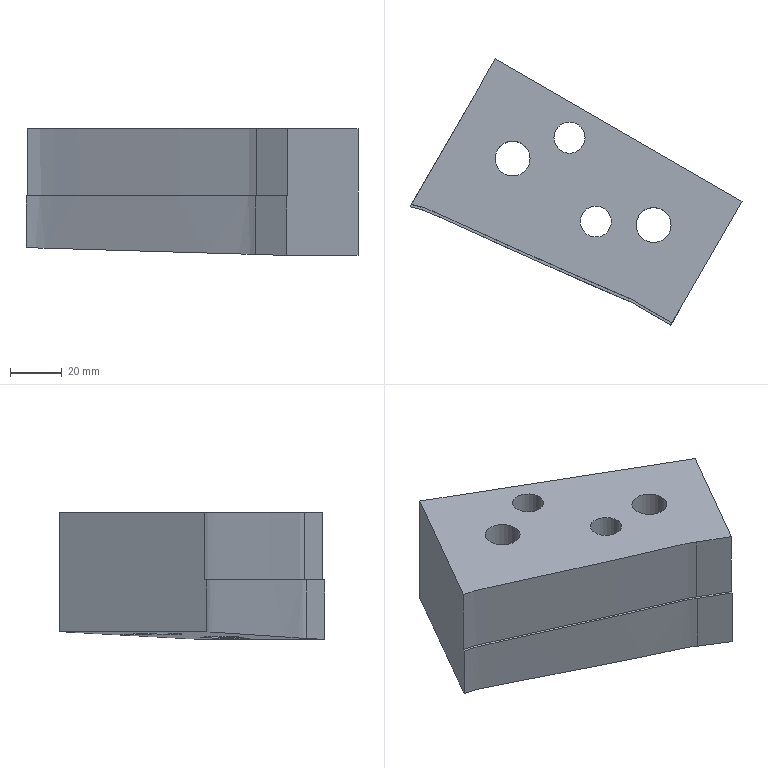Part | NX | features solid 2 | 1 solid | 22 faces | box 128.226 x 102.703 x 49 mm | volume 276802 mm3 | plane 12 | cylinder 8 | spline 2 | commonest cylinder face diameters 12 x2 13 x2 13.5 x2 19.5 x2
STEP:
#1=CARTESIAN_POINT('',(308.582,133.358,14.));
#2=VERTEX_POINT('',#1);
#3=CARTESIAN_POINT('',(397.207,94.712,14.));
#4=VERTEX_POINT('',#3);
#5=CARTESIAN_POINT('',(-190.231,-121.49,14.));
#6=CARTESIAN_POINT('',(-188.654,-121.152,14.));
#7=CARTESIAN_POINT('',(-185.47,-120.627,14.));
#8=CARTESIAN_POINT('',(-180.656,-120.141,14.));
#9=CARTESIAN_POINT('',(-175.882,-119.326,14.));
#10=CARTESIAN_POINT('',(-169.679,-117.528,14.));
#11=CARTESIAN_POINT('',(-162.185,-114.539,14.));
#12=CARTESIAN_POINT('',(-153.086,-111.254,14.));
#13=CARTESIAN_POINT('',(-144.031,-107.845,14.));
#14=CARTESIAN_POINT('',(-136.465,-105.061,14.));
#15=CARTESIAN_POINT('',(-130.418,-102.814,14.));
#16=CARTESIAN_POINT('',(-125.812,-101.329,14.));
#17=CARTESIAN_POINT('',(-121.306,-99.566,14.));
#18=CARTESIAN_POINT('',(-116.876,-97.626,14.));
#19=CARTESIAN_POINT('',(-112.335,-95.923,14.));
#20=CARTESIAN_POINT('',(-107.564,-95.05,14.));
#21=CARTESIAN_POINT('',(-102.756,-94.525,14.));
#22=CARTESIAN_POINT('',(-96.349,-93.771,14.));
#23=CARTESIAN_POINT('',(-89.902,-93.468,14.));
#24=CARTESIAN_POINT('',(-83.452,-93.448,14.));
#25=CARTESIAN_POINT('',(-77.002,-93.469,14.));
#26=CARTESIAN_POINT('',(-68.939,-93.411,14.));
#27=CARTESIAN_POINT('',(-56.04,-93.3,14.));
#28=CARTESIAN_POINT('',(-33.465,-93.184,14.));
#29=CARTESIAN_POINT('',(-7.666,-93.074,14.));
#30=CARTESIAN_POINT('',(14.907,-92.653,14.));
#31=CARTESIAN_POINT('',(27.794,-92.068,14.));
#32=CARTESIAN_POINT('',(40.668,-91.245,14.));
#33=CARTESIAN_POINT('',(51.917,-90.291,14.));
#34=CARTESIAN_POINT('',(61.528,-89.174,14.));
#35=CARTESIAN_POINT('',(67.939,-88.466,14.));
#36=CARTESIAN_POINT('',(79.125,-86.95,14.));
#37=CARTESIAN_POINT('',(95.161,-85.253,14.));
#38=CARTESIAN_POINT('',(114.404,-83.21,14.));
#39=CARTESIAN_POINT('',(133.568,-80.524,14.));
#40=CARTESIAN_POINT('',(152.734,-77.861,14.));
#41=CARTESIAN_POINT('',(171.916,-75.326,14.));
#42=CARTESIAN_POINT('',(191.055,-72.413,14.));
#43=CARTESIAN_POINT('',(207.17,-71.468,14.));
#44=CARTESIAN_POINT('',(219.951,-69.697,14.));
#45=CARTESIAN_POINT('',(232.724,-67.899,14.));
#46=CARTESIAN_POINT('',(248.708,-65.766,14.));
#47=CARTESIAN_POINT('',(267.87,-63.074,14.));
#48=CARTESIAN_POINT('',(287.038,-60.44,14.));
#49=CARTESIAN_POINT('',(301.448,-58.682,14.));
#50=CARTESIAN_POINT('',(310.976,-56.987,14.));
#51=CARTESIAN_POINT('',(314.916,-56.135,14.));
#52=CARTESIAN_POINT('',(318.052,-55.382,14.));
#53=CARTESIAN_POINT('',(320.39,-54.76,14.));
#54=CARTESIAN_POINT('',(322.686,-53.981,14.));
#55=CARTESIAN_POINT('',(325.595,-52.578,14.));
#56=CARTESIAN_POINT('',(328.769,-50.098,14.));
#57=CARTESIAN_POINT('',(332.247,-46.69,14.));
#58=CARTESIAN_POINT('',(335.795,-43.406,14.));
#59=CARTESIAN_POINT('',(343.661,-37.758,14.));
#60=CARTESIAN_POINT('',(355.164,-28.914,14.));
#61=CARTESIAN_POINT('',(370.422,-17.018,14.));
#62=CARTESIAN_POINT('',(383.264,-7.249,14.));
#63=CARTESIAN_POINT('',(392.416,-0.6713,14.));
#64=CARTESIAN_POINT('',(396.953,2.733,14.));
#65=CARTESIAN_POINT('',(398.886,5.372,14.));
#66=CARTESIAN_POINT('',(399.725,7.654,14.));
#67=CARTESIAN_POINT('',(399.76,10.078,14.));
#68=CARTESIAN_POINT('',(399.483,13.317,14.));
#69=CARTESIAN_POINT('',(399.712,17.34,14.));
#70=CARTESIAN_POINT('',(399.612,22.179,14.));
#71=CARTESIAN_POINT('',(399.633,31.854,14.));
#72=CARTESIAN_POINT('',(399.593,46.366,14.));
#73=CARTESIAN_POINT('',(399.637,62.491,14.));
#74=CARTESIAN_POINT('',(399.588,73.779,14.));
#75=CARTESIAN_POINT('',(399.652,79.422,14.));
#76=CARTESIAN_POINT('',(399.59,82.647,14.));
#77=CARTESIAN_POINT('',(399.564,85.065,14.));
#78=CARTESIAN_POINT('',(399.725,87.486,14.));
#79=CARTESIAN_POINT('',(399.756,89.902,14.));
#80=CARTESIAN_POINT('',(399.247,92.301,14.));
#81=CARTESIAN_POINT('',(397.362,95.008,14.));
#82=CARTESIAN_POINT('',(393.635,96.774,14.));
#83=CARTESIAN_POINT('',(389.279,98.826,14.));
#84=CARTESIAN_POINT('',(384.732,100.498,14.));
#85=CARTESIAN_POINT('',(378.765,102.95,14.));
#86=CARTESIAN_POINT('',(362.589,110.229,14.));
#87=CARTESIAN_POINT('',(344.928,118.135,14.));
#88=CARTESIAN_POINT('',(327.281,126.072,14.));
#89=CARTESIAN_POINT('',(319.932,129.381,14.));
#90=CARTESIAN_POINT('',(314.075,132.102,14.));
#91=CARTESIAN_POINT('',(309.387,133.376,14.));
#92=CARTESIAN_POINT('',(304.547,133.785,14.));
#93=CARTESIAN_POINT('',(299.716,133.401,14.));
#94=CARTESIAN_POINT('',(294.929,132.704,14.));
#95=CARTESIAN_POINT('',(288.543,131.8,14.));
#96=CARTESIAN_POINT('',(277.364,130.241,14.));
#97=CARTESIAN_POINT('',(242.2,125.552,14.));
#98=CARTESIAN_POINT('',(184.637,118.048,14.));
#99=CARTESIAN_POINT('',(120.701,109.541,14.));
#100=CARTESIAN_POINT('',(69.531,102.902,14.));
#101=CARTESIAN_POINT('',(40.777,98.94,14.));
#102=CARTESIAN_POINT('',(21.566,96.615,14.));
#103=CARTESIAN_POINT('',(8.743,95.212,14.));
#104=CARTESIAN_POINT('',(-7.301,93.575,14.));
#105=CARTESIAN_POINT('',(-26.625,92.505,14.));
#106=CARTESIAN_POINT('',(-45.971,92.017,14.));
#107=CARTESIAN_POINT('',(-62.09,91.675,14.));
#108=CARTESIAN_POINT('',(-74.987,91.256,14.));
#109=CARTESIAN_POINT('',(-84.664,91.165,14.));
#110=CARTESIAN_POINT('',(-94.319,91.781,14.));
#111=CARTESIAN_POINT('',(-103.929,92.966,14.));
#112=CARTESIAN_POINT('',(-113.495,94.403,14.));
#113=CARTESIAN_POINT('',(-119.856,95.492,14.));
#114=CARTESIAN_POINT('',(-122.997,96.222,14.));
#115=B_SPLINE_CURVE_WITH_KNOTS('',3,(#5,#6,#7,#8,#9,#10,#11,#12,#13,#14,#15,#16,#17,#18,#19,#20,#21,#22,#23,#24,#25,#26,#27,#28,#29,#30,#31,#32,#33,#34,#35,#36,#37,#38,#39,#40,#41,#42,#43,#44,#45,#46,#47,#48,#49,#50,#51,#52,#53,#54,#55,#56,#57,#58,#59,#60,#61,#62,#63,#64,#65,#66,#67,#68,#69,#70,#71,#72,#73,#74,#75,#76,#77,#78,#79,#80,#81,#82,#83,#84,#85,#86,#87,#88,#89,#90,#91,#92,#93,#94,#95,#96,#97,#98,#99,#100,#101,#102,#103,#104,#105,#106,#107,#108,#109,#110,#111,#112,#113,#114),.UNSPECIFIED.,.F.,.F.,(4,1,1,1,1,1,1,1,1,1,1,1,1,1,1,1,1,1,1,1,1,1,1,1,1,1,1,1,1,1,1,1,1,1,1,1,1,1,1,1,1,1,1,1,1,1,1,1,1,1,1,1,1,1,1,1,1,1,1,1,1,1,1,1,1,1,1,1,1,1,1,1,1,1,1,1,1,1,1,1,1,1,1,1,1,1,1,1,1,1,1,1,1,1,1,1,1,1,1,1,1,1,1,1,1,1,1,4),(0.4704,0.4724,0.4745,0.4766,0.4786,0.4828,0.4869,0.491,0.4952,0.4972,0.4993,0.5014,0.5035,0.5055,0.5076,0.5097,0.5117,0.5159,0.5179,0.52,0.5241,0.5283,0.5366,0.5531,0.5614,0.5655,0.5697,0.5779,0.58,0.5821,0.5862,0.5945,0.6028,0.611,0.6193,0.6276,0.6359,0.6441,0.6483,0.6524,0.6607,0.669,0.6772,0.6855,0.6876,0.6897,0.6907,0.6917,0.6928,0.6938,0.6959,0.6979,0.7,0.7021,0.7103,0.7186,0.7269,0.731,0.7331,0.7341,0.7352,0.7362,0.7372,0.7393,0.7414,0.7435,0.7517,0.76,0.7641,0.7662,0.7672,0.7683,0.7693,0.7703,0.7714,0.7724,0.7745,0.7766,0.7786,0.7807,0.7848,0.8014,0.8055,0.8097,0.8117,0.8138,0.8159,0.8179,0.82,0.8221,0.8262,0.8345,0.8676,0.9007,0.9172,0.9338,0.9379,0.9421,0.9503,0.9586,0.9669,0.9752,0.9793,0.9834,0.9876,0.9917,0.9959,1.),.UNSPECIFIED.);
#116=EDGE_CURVE('',#2,#4,#115,.F.);
#117=ORIENTED_EDGE('',*,*,#116,.F.);
#118=CARTESIAN_POINT('',(308.582,133.358,-6.));
#119=VERTEX_POINT('',#118);
#120=CARTESIAN_POINT('',(308.582,133.358,4.));
#121=DIRECTION('',(0.,0.,-1.));
#122=VECTOR('',#121,1000.);
#123=LINE('',#120,#122);
#124=EDGE_CURVE('',#119,#2,#123,.F.);
#125=ORIENTED_EDGE('',*,*,#124,.F.);
#126=CARTESIAN_POINT('',(397.207,94.712,-8.62));
#127=VERTEX_POINT('',#126);
#128=CARTESIAN_POINT('',(308.582,133.358,-6.));
#129=CARTESIAN_POINT('',(310.591,133.063,-6.051));
#130=CARTESIAN_POINT('',(314.461,132.008,-6.157));
#131=CARTESIAN_POINT('',(321.748,128.497,-6.377));
#132=CARTESIAN_POINT('',(330.972,124.433,-6.651));
#133=CARTESIAN_POINT('',(342.006,119.447,-6.979));
#134=CARTESIAN_POINT('',(353.053,114.5,-7.308));
#135=CARTESIAN_POINT('',(362.257,110.369,-7.581));
#136=CARTESIAN_POINT('',(369.619,107.065,-7.8));
#137=CARTESIAN_POINT('',(375.138,104.579,-7.964));
#138=CARTESIAN_POINT('',(380.676,102.138,-8.129));
#139=CARTESIAN_POINT('',(385.367,100.278,-8.265));
#140=CARTESIAN_POINT('',(389.141,98.841,-8.373));
#141=CARTESIAN_POINT('',(391.899,97.59,-8.456));
#142=CARTESIAN_POINT('',(394.641,96.327,-8.538));
#143=CARTESIAN_POINT('',(396.433,95.353,-8.593));
#144=CARTESIAN_POINT('',(397.207,94.712,-8.62));
#145=B_SPLINE_CURVE_WITH_KNOTS('',3,(#128,#129,#130,#131,#132,#133,#134,#135,#136,#137,#138,#139,#140,#141,#142,#143,#144),.UNSPECIFIED.,.F.,.F.,(4,1,1,1,1,1,1,1,1,1,1,1,1,1,4),(0.,0.006012,0.01202,0.02405,0.03607,0.0481,0.06012,0.06613,0.07214,0.07816,0.08417,0.08717,0.09018,0.09319,0.09619),.UNSPECIFIED.);
#146=EDGE_CURVE('',#119,#127,#145,.T.);
#147=ORIENTED_EDGE('',*,*,#146,.T.);
#148=CARTESIAN_POINT('',(397.207,94.712,15.353));
#149=DIRECTION('',(0.,0.,-1.));
#150=VECTOR('',#149,1000.);
#151=LINE('',#148,#150);
#152=EDGE_CURVE('',#127,#4,#151,.F.);
#153=ORIENTED_EDGE('',*,*,#152,.T.);
#154=EDGE_LOOP('',(#117,#125,#147,#153));
#155=FACE_BOUND('',#154,.T.);
#156=CARTESIAN_POINT('',(397.207,94.712,14.));
#157=CARTESIAN_POINT('',(397.207,94.712,-8.756));
#158=CARTESIAN_POINT('',(396.44,95.348,14.));
#159=CARTESIAN_POINT('',(396.44,95.348,-8.756));
#160=CARTESIAN_POINT('',(394.655,96.321,14.));
#161=CARTESIAN_POINT('',(394.655,96.321,-8.756));
#162=CARTESIAN_POINT('',(391.88,97.598,14.));
#163=CARTESIAN_POINT('',(391.88,97.598,-8.756));
#164=CARTESIAN_POINT('',(389.14,98.841,14.));
#165=CARTESIAN_POINT('',(389.14,98.841,-8.756));
#166=CARTESIAN_POINT('',(385.368,100.277,14.));
#167=CARTESIAN_POINT('',(385.368,100.277,-8.756));
#168=CARTESIAN_POINT('',(380.678,102.137,14.));
#169=CARTESIAN_POINT('',(380.678,102.137,-8.756));
#170=CARTESIAN_POINT('',(375.142,104.577,14.));
#171=CARTESIAN_POINT('',(375.142,104.577,-8.756));
#172=CARTESIAN_POINT('',(369.625,107.062,14.));
#173=CARTESIAN_POINT('',(369.625,107.062,-8.756));
#174=CARTESIAN_POINT('',(362.265,110.366,14.));
#175=CARTESIAN_POINT('',(362.265,110.366,-8.756));
#176=CARTESIAN_POINT('',(353.065,114.495,14.));
#177=CARTESIAN_POINT('',(353.065,114.495,-8.756));
#178=CARTESIAN_POINT('',(342.021,119.44,14.));
#179=CARTESIAN_POINT('',(342.021,119.44,-8.756));
#180=CARTESIAN_POINT('',(330.992,124.425,14.));
#181=CARTESIAN_POINT('',(330.992,124.425,-8.756));
#182=CARTESIAN_POINT('',(321.77,128.484,14.));
#183=CARTESIAN_POINT('',(321.77,128.484,-8.756));
#184=CARTESIAN_POINT('',(314.49,131.999,14.));
#185=CARTESIAN_POINT('',(314.49,131.999,-8.756));
#186=CARTESIAN_POINT('',(310.577,133.065,14.));
#187=CARTESIAN_POINT('',(310.577,133.065,-8.756));
#188=CARTESIAN_POINT('',(308.582,133.358,14.));
#189=CARTESIAN_POINT('',(308.582,133.358,-8.756));
#190=B_SPLINE_SURFACE_WITH_KNOTS('',3,1,((#156,#157),(#158,#159),(#160,#161),(#162,#163),(#164,#165),(#166,#167),(#168,#169),(#170,#171),(#172,#173),(#174,#175),(#176,#177),(#178,#179),(#180,#181),(#182,#183),(#184,#185),(#186,#187),(#188,#189)),.SURF_OF_LINEAR_EXTRUSION.,.F.,.F.,.F.,(4,1,1,1,1,1,1,1,1,1,1,1,1,1,4),(2,2),(0.7727,0.774,0.7753,0.7766,0.7779,0.7805,0.7831,0.7857,0.7883,0.7934,0.7986,0.8038,0.809,0.8115,0.8141),(0.,1.),.UNSPECIFIED.);
#191=ADVANCED_FACE('',(#155),#190,.T.);
#192=CARTESIAN_POINT('',(409.767,88.615,40.));
#193=VERTEX_POINT('',#192);
#194=CARTESIAN_POINT('',(397.778,95.537,40.));
#195=VERTEX_POINT('',#194);
#196=CARTESIAN_POINT('',(-185.99,432.575,40.));
#197=DIRECTION('',(-0.866,0.5,0.));
#198=VECTOR('',#197,1000.);
#199=LINE('',#196,#198);
#200=EDGE_CURVE('',#193,#195,#199,.T.);
#201=ORIENTED_EDGE('',*,*,#200,.F.);
#202=CARTESIAN_POINT('',(436.808,135.452,40.));
#203=VERTEX_POINT('',#202);
#204=CARTESIAN_POINT('',(180.279,-308.87,40.));
#205=DIRECTION('',(0.5,0.866,0.));
#206=VECTOR('',#205,1000.);
#207=LINE('',#204,#206);
#208=EDGE_CURVE('',#193,#203,#207,.T.);
#209=ORIENTED_EDGE('',*,*,#208,.T.);
#210=CARTESIAN_POINT('',(341.545,190.452,40.));
#211=VERTEX_POINT('',#210);
#212=CARTESIAN_POINT('',(-158.948,479.412,40.));
#213=DIRECTION('',(0.866,-0.5,0.));
#214=VECTOR('',#213,1000.);
#215=LINE('',#212,#214);
#216=EDGE_CURVE('',#211,#203,#215,.T.);
#217=ORIENTED_EDGE('',*,*,#216,.F.);
#218=CARTESIAN_POINT('',(309.118,134.287,40.));
#219=VERTEX_POINT('',#218);
#220=CARTESIAN_POINT('',(85.016,-253.87,40.));
#221=DIRECTION('',(0.5,0.866,0.));
#222=VECTOR('',#221,1000.);
#223=LINE('',#220,#222);
#224=EDGE_CURVE('',#219,#211,#223,.T.);
#225=ORIENTED_EDGE('',*,*,#224,.F.);
#226=CARTESIAN_POINT('',(397.778,95.537,40.));
#227=CARTESIAN_POINT('',(396.982,96.183,40.));
#228=CARTESIAN_POINT('',(395.223,97.16,40.));
#229=CARTESIAN_POINT('',(392.476,98.422,40.));
#230=CARTESIAN_POINT('',(389.726,99.681,40.));
#231=CARTESIAN_POINT('',(385.959,101.127,40.));
#232=CARTESIAN_POINT('',(381.266,102.971,40.));
#233=CARTESIAN_POINT('',(375.729,105.41,40.));
#234=CARTESIAN_POINT('',(370.211,107.895,40.));
#235=CARTESIAN_POINT('',(362.85,111.199,40.));
#236=CARTESIAN_POINT('',(353.649,115.329,40.));
#237=CARTESIAN_POINT('',(342.603,120.275,40.));
#238=CARTESIAN_POINT('',(331.573,125.26,40.));
#239=CARTESIAN_POINT('',(322.344,129.323,40.));
#240=CARTESIAN_POINT('',(315.069,132.831,40.));
#241=CARTESIAN_POINT('',(311.167,133.957,40.));
#242=CARTESIAN_POINT('',(309.118,134.287,40.));
#243=B_SPLINE_CURVE_WITH_KNOTS('',3,(#226,#227,#228,#229,#230,#231,#232,#233,#234,#235,#236,#237,#238,#239,#240,#241,#242),.UNSPECIFIED.,.F.,.F.,(4,1,1,1,1,1,1,1,1,1,1,1,1,1,4),(0.009262,0.01231,0.01537,0.01842,0.02147,0.02758,0.03368,0.03979,0.04589,0.0581,0.07031,0.08252,0.09473,0.1008,0.1069),.UNSPECIFIED.);
#244=EDGE_CURVE('',#195,#219,#243,.T.);
#245=ORIENTED_EDGE('',*,*,#244,.F.);
#246=EDGE_LOOP('',(#201,#209,#217,#225,#245));
#247=FACE_BOUND('',#246,.T.);
#248=CARTESIAN_POINT('',(386.337,127.641,40.));
#249=VERTEX_POINT('',#248);
#250=CARTESIAN_POINT('',(380.337,127.641,40.));
#251=DIRECTION('',(0.,0.,1.));
#252=DIRECTION('',(1.,0.,0.));
#253=AXIS2_PLACEMENT_3D('',#250,#251,#252);
#254=CIRCLE('',#253,6.);
#255=EDGE_CURVE('',#249,#249,#254,.T.);
#256=ORIENTED_EDGE('',*,*,#255,.F.);
#257=EDGE_LOOP('',(#256));
#258=FACE_BOUND('',#257,.T.);
#259=CARTESIAN_POINT('',(376.186,160.059,40.));
#260=VERTEX_POINT('',#259);
#261=CARTESIAN_POINT('',(370.186,160.059,40.));
#262=DIRECTION('',(0.,0.,1.));
#263=DIRECTION('',(1.,0.,0.));
#264=AXIS2_PLACEMENT_3D('',#261,#262,#263);
#265=CIRCLE('',#264,6.);
#266=EDGE_CURVE('',#260,#260,#265,.T.);
#267=ORIENTED_EDGE('',*,*,#266,.F.);
#268=EDGE_LOOP('',(#267));
#269=FACE_BOUND('',#268,.T.);
#270=CARTESIAN_POINT('',(409.407,126.301,40.));
#271=VERTEX_POINT('',#270);
#272=CARTESIAN_POINT('',(402.657,126.301,40.));
#273=DIRECTION('',(0.,0.,1.));
#274=DIRECTION('',(1.,0.,0.));
#275=AXIS2_PLACEMENT_3D('',#272,#273,#274);
#276=CIRCLE('',#275,6.75);
#277=EDGE_CURVE('',#271,#271,#276,.T.);
#278=ORIENTED_EDGE('',*,*,#277,.F.);
#279=EDGE_LOOP('',(#278));
#280=FACE_BOUND('',#279,.T.);
#281=CARTESIAN_POINT('',(354.946,151.971,40.));
#282=VERTEX_POINT('',#281);
#283=CARTESIAN_POINT('',(348.196,151.971,40.));
#284=DIRECTION('',(0.,0.,1.));
#285=DIRECTION('',(1.,0.,0.));
#286=AXIS2_PLACEMENT_3D('',#283,#284,#285);
#287=CIRCLE('',#286,6.75);
#288=EDGE_CURVE('',#282,#282,#287,.T.);
#289=ORIENTED_EDGE('',*,*,#288,.F.);
#290=EDGE_LOOP('',(#289));
#291=FACE_BOUND('',#290,.T.);
#292=CARTESIAN_POINT('',(-415.478,35.09,40.));
#293=DIRECTION('',(0.,0.,1.));
#294=DIRECTION('',(1.,0.,0.));
#295=AXIS2_PLACEMENT_3D('',#292,#293,#294);
#296=PLANE('',#295);
#297=ADVANCED_FACE('',(#247,#258,#269,#280,#291),#296,.T.);
#298=CARTESIAN_POINT('',(409.267,87.749,14.));
#299=VERTEX_POINT('',#298);
#300=CARTESIAN_POINT('',(409.767,88.615,14.));
#301=VERTEX_POINT('',#300);
#302=CARTESIAN_POINT('',(407.679,85.,14.));
#303=DIRECTION('',(0.5,0.866,0.));
#304=VECTOR('',#303,1000.);
#305=LINE('',#302,#304);
#306=EDGE_CURVE('',#299,#301,#305,.T.);
#307=ORIENTED_EDGE('',*,*,#306,.F.);
#308=CARTESIAN_POINT('',(409.267,87.749,-9.));
#309=VERTEX_POINT('',#308);
#310=CARTESIAN_POINT('',(409.267,87.749,2.));
#311=DIRECTION('',(0.,0.,1.));
#312=VECTOR('',#311,1000.);
#313=LINE('',#310,#312);
#314=EDGE_CURVE('',#309,#299,#313,.T.);
#315=ORIENTED_EDGE('',*,*,#314,.F.);
#316=CARTESIAN_POINT('',(436.808,135.452,-9.));
#317=VERTEX_POINT('',#316);
#318=CARTESIAN_POINT('',(55.229,-525.461,-9.));
#319=DIRECTION('',(-0.5,-0.866,0.));
#320=VECTOR('',#319,1000.);
#321=LINE('',#318,#320);
#322=EDGE_CURVE('',#317,#309,#321,.T.);
#323=ORIENTED_EDGE('',*,*,#322,.F.);
#324=CARTESIAN_POINT('',(436.808,135.452,2.));
#325=DIRECTION('',(0.,0.,-1.));
#326=VECTOR('',#325,1000.);
#327=LINE('',#324,#326);
#328=EDGE_CURVE('',#203,#317,#327,.T.);
#329=ORIENTED_EDGE('',*,*,#328,.F.);
#330=ORIENTED_EDGE('',*,*,#208,.F.);
#331=CARTESIAN_POINT('',(409.767,88.615,2.));
#332=DIRECTION('',(0.,0.,1.));
#333=VECTOR('',#332,1000.);
#334=LINE('',#331,#333);
#335=EDGE_CURVE('',#301,#193,#334,.T.);
#336=ORIENTED_EDGE('',*,*,#335,.F.);
#337=EDGE_LOOP('',(#307,#315,#323,#329,#330,#336));
#338=FACE_BOUND('',#337,.T.);
#339=CARTESIAN_POINT('',(407.679,85.,2.));
#340=DIRECTION('',(0.866,-0.5,0.));
#341=DIRECTION('',(0.5,0.866,0.));
#342=AXIS2_PLACEMENT_3D('',#339,#340,#341);
#343=PLANE('',#342);
#344=ADVANCED_FACE('',(#338),#343,.T.);
#345=ORIENTED_EDGE('',*,*,#328,.T.);
#346=CARTESIAN_POINT('',(341.545,190.452,-6.));
#347=VERTEX_POINT('',#346);
#348=CARTESIAN_POINT('',(-88.483,438.729,7.542));
#349=DIRECTION('',(-0.8657,0.4998,0.02726));
#350=VECTOR('',#349,1000.);
#351=LINE('',#348,#350);
#352=EDGE_CURVE('',#317,#347,#351,.T.);
#353=ORIENTED_EDGE('',*,*,#352,.T.);
#354=CARTESIAN_POINT('',(341.545,190.452,2.));
#355=DIRECTION('',(0.,0.,1.));
#356=VECTOR('',#355,1000.);
#357=LINE('',#354,#356);
#358=EDGE_CURVE('',#347,#211,#357,.T.);
#359=ORIENTED_EDGE('',*,*,#358,.T.);
#360=ORIENTED_EDGE('',*,*,#216,.T.);
#361=EDGE_LOOP('',(#345,#353,#359,#360));
#362=FACE_BOUND('',#361,.T.);
#363=CARTESIAN_POINT('',(400.854,156.21,2.));
#364=DIRECTION('',(-0.5,-0.866,0.));
#365=DIRECTION('',(0.866,-0.5,0.));
#366=AXIS2_PLACEMENT_3D('',#363,#364,#365);
#367=PLANE('',#366);
#368=ADVANCED_FACE('',(#362),#367,.F.);
#369=ORIENTED_EDGE('',*,*,#124,.T.);
#370=CARTESIAN_POINT('',(309.118,134.287,14.));
#371=VERTEX_POINT('',#370);
#372=CARTESIAN_POINT('',(326.746,164.819,14.));
#373=DIRECTION('',(0.5,0.866,0.));
#374=VECTOR('',#373,1000.);
#375=LINE('',#372,#374);
#376=EDGE_CURVE('',#2,#371,#375,.T.);
#377=ORIENTED_EDGE('',*,*,#376,.T.);
#378=CARTESIAN_POINT('',(309.118,134.287,57.));
#379=DIRECTION('',(0.,0.,1.));
#380=VECTOR('',#379,1000.);
#381=LINE('',#378,#380);
#382=EDGE_CURVE('',#371,#219,#381,.T.);
#383=ORIENTED_EDGE('',*,*,#382,.T.);
#384=ORIENTED_EDGE('',*,*,#224,.T.);
#385=ORIENTED_EDGE('',*,*,#358,.F.);
#386=CARTESIAN_POINT('',(-40.033,-470.461,-6.));
#387=DIRECTION('',(-0.5,-0.866,0.));
#388=VECTOR('',#387,1000.);
#389=LINE('',#386,#388);
#390=EDGE_CURVE('',#347,#119,#389,.T.);
#391=ORIENTED_EDGE('',*,*,#390,.T.);
#392=EDGE_LOOP('',(#369,#377,#383,#384,#385,#391));
#393=FACE_BOUND('',#392,.T.);
#394=CARTESIAN_POINT('',(326.746,164.819,23.));
#395=DIRECTION('',(0.866,-0.5,0.));
#396=DIRECTION('',(0.5,0.866,0.));
#397=AXIS2_PLACEMENT_3D('',#394,#395,#396);
#398=PLANE('',#397);
#399=ADVANCED_FACE('',(#393),#398,.F.);
#400=ORIENTED_EDGE('',*,*,#288,.T.);
#401=EDGE_LOOP('',(#400));
#402=FACE_BOUND('',#401,.T.);
#403=CARTESIAN_POINT('',(354.946,151.971,9.));
#404=VERTEX_POINT('',#403);
#405=CARTESIAN_POINT('',(348.196,151.971,9.));
#406=DIRECTION('',(0.,0.,1.));
#407=DIRECTION('',(1.,0.,0.));
#408=AXIS2_PLACEMENT_3D('',#405,#406,#407);
#409=CIRCLE('',#408,6.75);
#410=EDGE_CURVE('',#404,#404,#409,.T.);
#411=ORIENTED_EDGE('',*,*,#410,.F.);
#412=EDGE_LOOP('',(#411));
#413=FACE_BOUND('',#412,.T.);
#414=CARTESIAN_POINT('',(348.196,151.971,94.));
#415=DIRECTION('',(0.,0.,1.));
#416=DIRECTION('',(1.,0.,0.));
#417=AXIS2_PLACEMENT_3D('',#414,#415,#416);
#418=CYLINDRICAL_SURFACE('',#417,6.75);
#419=ADVANCED_FACE('',(#402,#413),#418,.F.);
#420=ORIENTED_EDGE('',*,*,#410,.T.);
#421=EDGE_LOOP('',(#420));
#422=FACE_BOUND('',#421,.T.);
#423=CARTESIAN_POINT('',(357.946,151.971,9.));
#424=VERTEX_POINT('',#423);
#425=CARTESIAN_POINT('',(348.196,151.971,9.));
#426=DIRECTION('',(0.,0.,1.));
#427=DIRECTION('',(1.,0.,0.));
#428=AXIS2_PLACEMENT_3D('',#425,#426,#427);
#429=CIRCLE('',#428,9.75);
#430=EDGE_CURVE('',#424,#424,#429,.T.);
#431=ORIENTED_EDGE('',*,*,#430,.F.);
#432=EDGE_LOOP('',(#431));
#433=FACE_BOUND('',#432,.T.);
#434=CARTESIAN_POINT('',(348.196,151.971,9.));
#435=DIRECTION('',(0.,0.,1.));
#436=DIRECTION('',(1.,0.,0.));
#437=AXIS2_PLACEMENT_3D('',#434,#435,#436);
#438=PLANE('',#437);
#439=ADVANCED_FACE('',(#422,#433),#438,.F.);
#440=ORIENTED_EDGE('',*,*,#430,.T.);
#441=EDGE_LOOP('',(#440));
#442=FACE_BOUND('',#441,.T.);
#443=CARTESIAN_POINT('',(356.639,147.096,-6.948));
#444=VERTEX_POINT('',#443);
#445=CARTESIAN_POINT('',(348.196,151.971,-6.682));
#446=DIRECTION('',(0.02361,-0.01363,0.9996));
#447=DIRECTION('',(0.8657,-0.4998,-0.02726));
#448=AXIS2_PLACEMENT_3D('',#445,#446,#447);
#449=ELLIPSE('',#448,9.754,9.75);
#450=EDGE_CURVE('',#444,#444,#449,.T.);
#451=ORIENTED_EDGE('',*,*,#450,.F.);
#452=EDGE_LOOP('',(#451));
#453=FACE_BOUND('',#452,.T.);
#454=CARTESIAN_POINT('',(348.196,151.971,-6.));
#455=DIRECTION('',(0.,0.,1.));
#456=DIRECTION('',(1.,0.,0.));
#457=AXIS2_PLACEMENT_3D('',#454,#455,#456);
#458=CYLINDRICAL_SURFACE('',#457,9.75);
#459=ADVANCED_FACE('',(#442,#453),#458,.F.);
#460=ORIENTED_EDGE('',*,*,#277,.T.);
#461=EDGE_LOOP('',(#460));
#462=FACE_BOUND('',#461,.T.);
#463=CARTESIAN_POINT('',(409.407,126.301,9.));
#464=VERTEX_POINT('',#463);
#465=CARTESIAN_POINT('',(402.657,126.301,9.));
#466=DIRECTION('',(0.,0.,1.));
#467=DIRECTION('',(1.,0.,0.));
#468=AXIS2_PLACEMENT_3D('',#465,#466,#467);
#469=CIRCLE('',#468,6.75);
#470=EDGE_CURVE('',#464,#464,#469,.T.);
#471=ORIENTED_EDGE('',*,*,#470,.F.);
#472=EDGE_LOOP('',(#471));
#473=FACE_BOUND('',#472,.T.);
#474=CARTESIAN_POINT('',(402.657,126.301,94.));
#475=DIRECTION('',(0.,0.,1.));
#476=DIRECTION('',(1.,0.,0.));
#477=AXIS2_PLACEMENT_3D('',#474,#475,#476);
#478=CYLINDRICAL_SURFACE('',#477,6.75);
#479=ADVANCED_FACE('',(#462,#473),#478,.F.);
#480=ORIENTED_EDGE('',*,*,#470,.T.);
#481=EDGE_LOOP('',(#480));
#482=FACE_BOUND('',#481,.T.);
#483=CARTESIAN_POINT('',(412.407,126.301,9.));
#484=VERTEX_POINT('',#483);
#485=CARTESIAN_POINT('',(402.657,126.301,9.));
#486=DIRECTION('',(0.,0.,1.));
#487=DIRECTION('',(1.,0.,0.));
#488=AXIS2_PLACEMENT_3D('',#485,#486,#487);
#489=CIRCLE('',#488,9.75);
#490=EDGE_CURVE('',#484,#484,#489,.T.);
#491=ORIENTED_EDGE('',*,*,#490,.F.);
#492=EDGE_LOOP('',(#491));
#493=FACE_BOUND('',#492,.T.);
#494=CARTESIAN_POINT('',(402.657,126.301,9.));
#495=DIRECTION('',(0.,0.,1.));
#496=DIRECTION('',(1.,0.,0.));
#497=AXIS2_PLACEMENT_3D('',#494,#495,#496);
#498=PLANE('',#497);
#499=ADVANCED_FACE('',(#482,#493),#498,.F.);
#500=ORIENTED_EDGE('',*,*,#490,.T.);
#501=EDGE_LOOP('',(#500));
#502=FACE_BOUND('',#501,.T.);
#503=CARTESIAN_POINT('',(411.101,121.426,-8.584));
#504=VERTEX_POINT('',#503);
#505=CARTESIAN_POINT('',(402.657,126.301,-8.318));
#506=DIRECTION('',(0.02361,-0.01363,0.9996));
#507=DIRECTION('',(0.8657,-0.4998,-0.02726));
#508=AXIS2_PLACEMENT_3D('',#505,#506,#507);
#509=ELLIPSE('',#508,9.754,9.75);
#510=EDGE_CURVE('',#504,#504,#509,.T.);
#511=ORIENTED_EDGE('',*,*,#510,.F.);
#512=EDGE_LOOP('',(#511));
#513=FACE_BOUND('',#512,.T.);
#514=CARTESIAN_POINT('',(402.657,126.301,-6.));
#515=DIRECTION('',(0.,0.,1.));
#516=DIRECTION('',(1.,0.,0.));
#517=AXIS2_PLACEMENT_3D('',#514,#515,#516);
#518=CYLINDRICAL_SURFACE('',#517,9.75);
#519=ADVANCED_FACE('',(#502,#513),#518,.F.);
#520=ORIENTED_EDGE('',*,*,#266,.T.);
#521=EDGE_LOOP('',(#520));
#522=FACE_BOUND('',#521,.T.);
#523=CARTESIAN_POINT('',(376.186,160.059,14.));
#524=VERTEX_POINT('',#523);
#525=CARTESIAN_POINT('',(370.186,160.059,14.));
#526=DIRECTION('',(0.,0.,1.));
#527=DIRECTION('',(1.,0.,0.));
#528=AXIS2_PLACEMENT_3D('',#525,#526,#527);
#529=CIRCLE('',#528,6.);
#530=EDGE_CURVE('',#524,#524,#529,.T.);
#531=ORIENTED_EDGE('',*,*,#530,.F.);
#532=EDGE_LOOP('',(#531));
#533=FACE_BOUND('',#532,.T.);
#534=CARTESIAN_POINT('',(370.186,160.059,94.));
#535=DIRECTION('',(0.,0.,1.));
#536=DIRECTION('',(1.,0.,0.));
#537=AXIS2_PLACEMENT_3D('',#534,#535,#536);
#538=CYLINDRICAL_SURFACE('',#537,6.);
#539=ADVANCED_FACE('',(#522,#533),#538,.F.);
#540=ORIENTED_EDGE('',*,*,#530,.T.);
#541=EDGE_LOOP('',(#540));
#542=FACE_BOUND('',#541,.T.);
#543=CARTESIAN_POINT('',(376.686,160.059,14.));
#544=VERTEX_POINT('',#543);
#545=CARTESIAN_POINT('',(370.186,160.059,14.));
#546=DIRECTION('',(0.,0.,1.));
#547=DIRECTION('',(1.,0.,0.));
#548=AXIS2_PLACEMENT_3D('',#545,#546,#547);
#549=CIRCLE('',#548,6.5);
#550=EDGE_CURVE('',#544,#544,#549,.T.);
#551=ORIENTED_EDGE('',*,*,#550,.F.);
#552=EDGE_LOOP('',(#551));
#553=FACE_BOUND('',#552,.T.);
#554=CARTESIAN_POINT('',(370.186,160.059,14.));
#555=DIRECTION('',(0.,0.,1.));
#556=DIRECTION('',(1.,0.,0.));
#557=AXIS2_PLACEMENT_3D('',#554,#555,#556);
#558=PLANE('',#557);
#559=ADVANCED_FACE('',(#542,#553),#558,.F.);
#560=ORIENTED_EDGE('',*,*,#550,.T.);
#561=EDGE_LOOP('',(#560));
#562=FACE_BOUND('',#561,.T.);
#563=CARTESIAN_POINT('',(375.815,156.809,-7.268));
#564=VERTEX_POINT('',#563);
#565=CARTESIAN_POINT('',(370.186,160.059,-7.091));
#566=DIRECTION('',(0.02361,-0.01363,0.9996));
#567=DIRECTION('',(0.8657,-0.4998,-0.02726));
#568=AXIS2_PLACEMENT_3D('',#565,#566,#567);
#569=ELLIPSE('',#568,6.502,6.5);
#570=EDGE_CURVE('',#564,#564,#569,.T.);
#571=ORIENTED_EDGE('',*,*,#570,.F.);
#572=EDGE_LOOP('',(#571));
#573=FACE_BOUND('',#572,.T.);
#574=CARTESIAN_POINT('',(370.186,160.059,-6.));
#575=DIRECTION('',(0.,0.,1.));
#576=DIRECTION('',(1.,0.,0.));
#577=AXIS2_PLACEMENT_3D('',#574,#575,#576);
#578=CYLINDRICAL_SURFACE('',#577,6.5);
#579=ADVANCED_FACE('',(#562,#573),#578,.F.);
#580=ORIENTED_EDGE('',*,*,#255,.T.);
#581=EDGE_LOOP('',(#580));
#582=FACE_BOUND('',#581,.T.);
#583=CARTESIAN_POINT('',(386.337,127.641,14.));
#584=VERTEX_POINT('',#583);
#585=CARTESIAN_POINT('',(380.337,127.641,14.));
#586=DIRECTION('',(0.,0.,1.));
#587=DIRECTION('',(1.,0.,0.));
#588=AXIS2_PLACEMENT_3D('',#585,#586,#587);
#589=CIRCLE('',#588,6.);
#590=EDGE_CURVE('',#584,#584,#589,.T.);
#591=ORIENTED_EDGE('',*,*,#590,.F.);
#592=EDGE_LOOP('',(#591));
#593=FACE_BOUND('',#592,.T.);
#594=CARTESIAN_POINT('',(380.337,127.641,94.));
#595=DIRECTION('',(0.,0.,1.));
#596=DIRECTION('',(1.,0.,0.));
#597=AXIS2_PLACEMENT_3D('',#594,#595,#596);
#598=CYLINDRICAL_SURFACE('',#597,6.);
#599=ADVANCED_FACE('',(#582,#593),#598,.F.);
#600=ORIENTED_EDGE('',*,*,#590,.T.);
#601=EDGE_LOOP('',(#600));
#602=FACE_BOUND('',#601,.T.);
#603=CARTESIAN_POINT('',(386.837,127.641,14.));
#604=VERTEX_POINT('',#603);
#605=CARTESIAN_POINT('',(380.337,127.641,14.));
#606=DIRECTION('',(0.,0.,1.));
#607=DIRECTION('',(1.,0.,0.));
#608=AXIS2_PLACEMENT_3D('',#605,#606,#607);
#609=CIRCLE('',#608,6.5);
#610=EDGE_CURVE('',#604,#604,#609,.T.);
#611=ORIENTED_EDGE('',*,*,#610,.F.);
#612=EDGE_LOOP('',(#611));
#613=FACE_BOUND('',#612,.T.);
#614=CARTESIAN_POINT('',(380.337,127.641,14.));
#615=DIRECTION('',(0.,0.,1.));
#616=DIRECTION('',(1.,0.,0.));
#617=AXIS2_PLACEMENT_3D('',#614,#615,#616);
#618=PLANE('',#617);
#619=ADVANCED_FACE('',(#602,#613),#618,.F.);
#620=ORIENTED_EDGE('',*,*,#610,.T.);
#621=EDGE_LOOP('',(#620));
#622=FACE_BOUND('',#621,.T.);
#623=CARTESIAN_POINT('',(385.966,124.391,-7.95));
#624=VERTEX_POINT('',#623);
#625=CARTESIAN_POINT('',(380.337,127.641,-7.773));
#626=DIRECTION('',(0.02361,-0.01363,0.9996));
#627=DIRECTION('',(0.8657,-0.4998,-0.02726));
#628=AXIS2_PLACEMENT_3D('',#625,#626,#627);
#629=ELLIPSE('',#628,6.502,6.5);
#630=EDGE_CURVE('',#624,#624,#629,.T.);
#631=ORIENTED_EDGE('',*,*,#630,.F.);
#632=EDGE_LOOP('',(#631));
#633=FACE_BOUND('',#632,.T.);
#634=CARTESIAN_POINT('',(380.337,127.641,-6.));
#635=DIRECTION('',(0.,0.,1.));
#636=DIRECTION('',(1.,0.,0.));
#637=AXIS2_PLACEMENT_3D('',#634,#635,#636);
#638=CYLINDRICAL_SURFACE('',#637,6.5);
#639=ADVANCED_FACE('',(#622,#633),#638,.F.);
#640=ORIENTED_EDGE('',*,*,#630,.T.);
#641=EDGE_LOOP('',(#640));
#642=FACE_BOUND('',#641,.T.);
#643=ORIENTED_EDGE('',*,*,#570,.T.);
#644=EDGE_LOOP('',(#643));
#645=FACE_BOUND('',#644,.T.);
#646=ORIENTED_EDGE('',*,*,#510,.T.);
#647=EDGE_LOOP('',(#646));
#648=FACE_BOUND('',#647,.T.);
#649=ORIENTED_EDGE('',*,*,#450,.T.);
#650=EDGE_LOOP('',(#649));
#651=FACE_BOUND('',#650,.T.);
#652=ORIENTED_EDGE('',*,*,#322,.T.);
#653=CARTESIAN_POINT('',(314.004,142.749,-6.));
#654=DIRECTION('',(-0.8657,0.4998,0.02726));
#655=VECTOR('',#654,1000.);
#656=LINE('',#653,#655);
#657=EDGE_CURVE('',#309,#127,#656,.T.);
#658=ORIENTED_EDGE('',*,*,#657,.T.);
#659=ORIENTED_EDGE('',*,*,#146,.F.);
#660=ORIENTED_EDGE('',*,*,#390,.F.);
#661=ORIENTED_EDGE('',*,*,#352,.F.);
#662=EDGE_LOOP('',(#652,#658,#659,#660,#661));
#663=FACE_BOUND('',#662,.T.);
#664=CARTESIAN_POINT('',(341.545,190.452,-6.));
#665=DIRECTION('',(0.02361,-0.01363,0.9996));
#666=DIRECTION('',(0.9997,0.,-0.02361));
#667=AXIS2_PLACEMENT_3D('',#664,#665,#666);
#668=PLANE('',#667);
#669=ADVANCED_FACE('',(#642,#645,#648,#651,#663),#668,.F.);
#670=ORIENTED_EDGE('',*,*,#314,.T.);
#671=CARTESIAN_POINT('',(393.655,96.763,14.));
#672=DIRECTION('',(-0.866,0.5,0.));
#673=VECTOR('',#672,1000.);
#674=LINE('',#671,#673);
#675=EDGE_CURVE('',#299,#4,#674,.T.);
#676=ORIENTED_EDGE('',*,*,#675,.T.);
#677=ORIENTED_EDGE('',*,*,#152,.F.);
#678=ORIENTED_EDGE('',*,*,#657,.F.);
#679=EDGE_LOOP('',(#670,#676,#677,#678));
#680=FACE_BOUND('',#679,.T.);
#681=CARTESIAN_POINT('',(393.655,96.763,100.));
#682=DIRECTION('',(0.5,0.866,0.));
#683=DIRECTION('',(-0.866,0.5,0.));
#684=AXIS2_PLACEMENT_3D('',#681,#682,#683);
#685=PLANE('',#684);
#686=ADVANCED_FACE('',(#680),#685,.F.);
#687=ORIENTED_EDGE('',*,*,#116,.T.);
#688=ORIENTED_EDGE('',*,*,#675,.F.);
#689=ORIENTED_EDGE('',*,*,#306,.T.);
#690=CARTESIAN_POINT('',(397.778,95.537,14.));
#691=VERTEX_POINT('',#690);
#692=CARTESIAN_POINT('',(409.767,88.615,14.));
#693=DIRECTION('',(-0.866,0.5,0.));
#694=VECTOR('',#693,1000.);
#695=LINE('',#692,#694);
#696=EDGE_CURVE('',#301,#691,#695,.T.);
#697=ORIENTED_EDGE('',*,*,#696,.T.);
#698=CARTESIAN_POINT('',(397.778,95.537,14.));
#699=CARTESIAN_POINT('',(396.913,96.239,14.));
#700=CARTESIAN_POINT('',(394.998,97.263,14.));
#701=CARTESIAN_POINT('',(392.27,98.52,14.));
#702=CARTESIAN_POINT('',(389.486,99.781,14.));
#703=CARTESIAN_POINT('',(385.694,101.223,14.));
#704=CARTESIAN_POINT('',(381.084,103.052,14.));
#705=CARTESIAN_POINT('',(375.583,105.475,14.));
#706=CARTESIAN_POINT('',(370.095,107.947,14.));
#707=CARTESIAN_POINT('',(362.769,111.236,14.));
#708=CARTESIAN_POINT('',(353.612,115.343,14.));
#709=CARTESIAN_POINT('',(342.624,120.273,14.));
#710=CARTESIAN_POINT('',(333.469,124.381,14.));
#711=CARTESIAN_POINT('',(326.15,127.685,14.));
#712=CARTESIAN_POINT('',(320.659,130.125,14.));
#713=CARTESIAN_POINT('',(315.224,132.777,14.));
#714=CARTESIAN_POINT('',(311.174,133.956,14.));
#715=CARTESIAN_POINT('',(309.118,134.287,14.));
#716=B_SPLINE_CURVE_WITH_KNOTS('',3,(#698,#699,#700,#701,#702,#703,#704,#705,#706,#707,#708,#709,#710,#711,#712,#713,#714,#715),.UNSPECIFIED.,.F.,.F.,(4,1,1,1,1,1,1,1,1,1,1,1,1,1,1,4),(0.7728,0.7741,0.7753,0.7766,0.7779,0.7805,0.7831,0.7856,0.7882,0.7934,0.7985,0.8037,0.8062,0.8088,0.8114,0.814),.UNSPECIFIED.);
#717=EDGE_CURVE('',#691,#371,#716,.T.);
#718=ORIENTED_EDGE('',*,*,#717,.T.);
#719=ORIENTED_EDGE('',*,*,#376,.F.);
#720=EDGE_LOOP('',(#687,#688,#689,#697,#718,#719));
#721=FACE_BOUND('',#720,.T.);
#722=CARTESIAN_POINT('',(-190.231,-121.49,14.));
#723=DIRECTION('',(0.,0.,-1.));
#724=DIRECTION('',(-1.,0.,0.));
#725=AXIS2_PLACEMENT_3D('',#722,#723,#724);
#726=PLANE('',#725);
#727=ADVANCED_FACE('',(#721),#726,.F.);
#728=ORIENTED_EDGE('',*,*,#717,.F.);
#729=CARTESIAN_POINT('',(397.778,95.537,27.));
#730=DIRECTION('',(0.,0.,1.));
#731=VECTOR('',#730,1000.);
#732=LINE('',#729,#731);
#733=EDGE_CURVE('',#691,#195,#732,.T.);
#734=ORIENTED_EDGE('',*,*,#733,.T.);
#735=ORIENTED_EDGE('',*,*,#244,.T.);
#736=ORIENTED_EDGE('',*,*,#382,.F.);
#737=EDGE_LOOP('',(#728,#734,#735,#736));
#738=FACE_BOUND('',#737,.T.);
#739=CARTESIAN_POINT('',(397.778,95.537,14.));
#740=CARTESIAN_POINT('',(397.778,95.537,40.));
#741=CARTESIAN_POINT('',(396.913,96.239,14.));
#742=CARTESIAN_POINT('',(396.913,96.239,40.));
#743=CARTESIAN_POINT('',(394.998,97.263,14.));
#744=CARTESIAN_POINT('',(394.998,97.263,40.));
#745=CARTESIAN_POINT('',(392.27,98.52,14.));
#746=CARTESIAN_POINT('',(392.27,98.52,40.));
#747=CARTESIAN_POINT('',(389.486,99.781,14.));
#748=CARTESIAN_POINT('',(389.486,99.781,40.));
#749=CARTESIAN_POINT('',(385.694,101.223,14.));
#750=CARTESIAN_POINT('',(385.694,101.223,40.));
#751=CARTESIAN_POINT('',(381.084,103.052,14.));
#752=CARTESIAN_POINT('',(381.084,103.052,40.));
#753=CARTESIAN_POINT('',(375.583,105.475,14.));
#754=CARTESIAN_POINT('',(375.583,105.475,40.));
#755=CARTESIAN_POINT('',(370.095,107.947,14.));
#756=CARTESIAN_POINT('',(370.095,107.947,40.));
#757=CARTESIAN_POINT('',(362.769,111.236,14.));
#758=CARTESIAN_POINT('',(362.769,111.236,40.));
#759=CARTESIAN_POINT('',(353.612,115.343,14.));
#760=CARTESIAN_POINT('',(353.612,115.343,40.));
#761=CARTESIAN_POINT('',(342.624,120.273,14.));
#762=CARTESIAN_POINT('',(342.624,120.273,40.));
#763=CARTESIAN_POINT('',(333.469,124.381,14.));
#764=CARTESIAN_POINT('',(333.469,124.381,40.));
#765=CARTESIAN_POINT('',(326.15,127.685,14.));
#766=CARTESIAN_POINT('',(326.15,127.685,40.));
#767=CARTESIAN_POINT('',(320.659,130.125,14.));
#768=CARTESIAN_POINT('',(320.659,130.125,40.));
#769=CARTESIAN_POINT('',(315.224,132.777,14.));
#770=CARTESIAN_POINT('',(315.224,132.777,40.));
#771=CARTESIAN_POINT('',(311.174,133.956,14.));
#772=CARTESIAN_POINT('',(311.174,133.956,40.));
#773=CARTESIAN_POINT('',(309.118,134.287,14.));
#774=CARTESIAN_POINT('',(309.118,134.287,40.));
#775=B_SPLINE_SURFACE_WITH_KNOTS('',3,1,((#739,#740),(#741,#742),(#743,#744),(#745,#746),(#747,#748),(#749,#750),(#751,#752),(#753,#754),(#755,#756),(#757,#758),(#759,#760),(#761,#762),(#763,#764),(#765,#766),(#767,#768),(#769,#770),(#771,#772),(#773,#774)),.SURF_OF_LINEAR_EXTRUSION.,.F.,.F.,.F.,(4,1,1,1,1,1,1,1,1,1,1,1,1,1,1,4),(2,2),(0.7728,0.7741,0.7753,0.7766,0.7779,0.7805,0.7831,0.7856,0.7882,0.7934,0.7985,0.8037,0.8062,0.8088,0.8114,0.814),(0.,1.),.UNSPECIFIED.);
#776=ADVANCED_FACE('',(#738),#775,.F.);
#777=ORIENTED_EDGE('',*,*,#335,.T.);
#778=ORIENTED_EDGE('',*,*,#200,.T.);
#779=ORIENTED_EDGE('',*,*,#733,.F.);
#780=ORIENTED_EDGE('',*,*,#696,.F.);
#781=EDGE_LOOP('',(#777,#778,#779,#780));
#782=FACE_BOUND('',#781,.T.);
#783=CARTESIAN_POINT('',(409.767,88.615,11.));
#784=DIRECTION('',(0.5,0.866,0.));
#785=DIRECTION('',(-0.866,0.5,0.));
#786=AXIS2_PLACEMENT_3D('',#783,#784,#785);
#787=PLANE('',#786);
#788=ADVANCED_FACE('',(#782),#787,.F.);
#789=CLOSED_SHELL('',(#191,#297,#344,#368,#399,#419,#439,#459,#479,#499,#519,#539,#559,#579,#599,#619,#639,#669,#686,#727,#776,#788));
#790=MANIFOLD_SOLID_BREP('',#789);
#791=(LENGTH_UNIT()NAMED_UNIT(*)SI_UNIT(.MILLI.,.METRE.));
#792=UNCERTAINTY_MEASURE_WITH_UNIT(LENGTH_MEASURE(0.0508),#791,'','');
#793=(NAMED_UNIT(*)PLANE_ANGLE_UNIT()SI_UNIT($,.RADIAN.));
#794=(NAMED_UNIT(*)SI_UNIT($,.STERADIAN.)SOLID_ANGLE_UNIT());
#795=(GEOMETRIC_REPRESENTATION_CONTEXT(3)GLOBAL_UNCERTAINTY_ASSIGNED_CONTEXT((#792))GLOBAL_UNIT_ASSIGNED_CONTEXT((#791,#793,#794))REPRESENTATION_CONTEXT('',''));
#796=ADVANCED_BREP_SHAPE_REPRESENTATION('',(#790),#795);